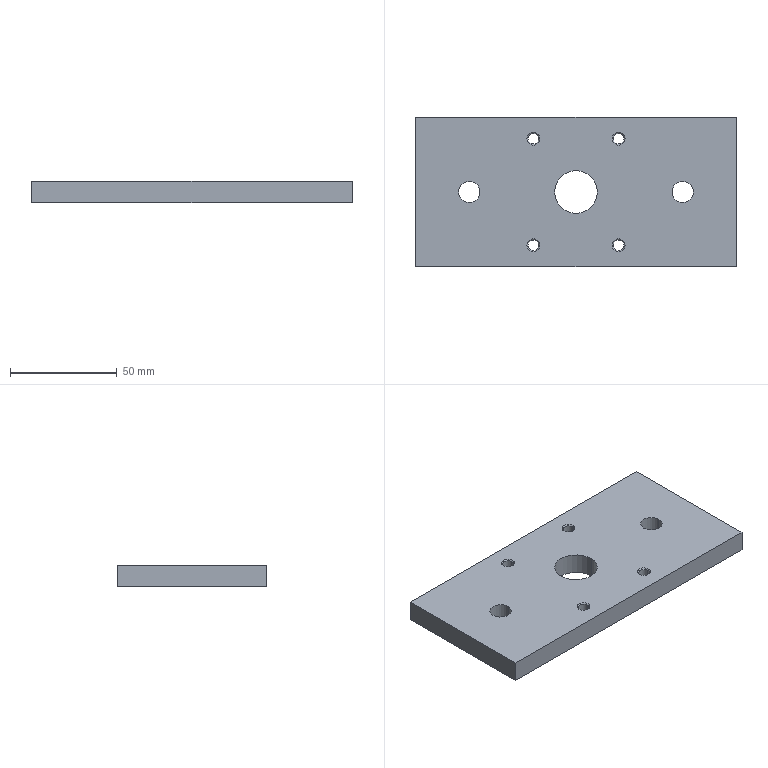Part | SolidWorks | features Cut 2, Extrusion 1, HoleWzd 1 | 1 solid | 28 faces | box 150 x 70 x 10 mm | volume 99493 mm3 | cylinder 14 | cone 8 | plane 6 | commonest cylinder face diameters 5 x8 10 x4 20 x2
STEP:
#1=CARTESIAN_POINT('',(17.5,25.,9.475));
#2=VERTEX_POINT('',#1);
#3=CARTESIAN_POINT('',(22.5,25.,9.475));
#4=VERTEX_POINT('',#3);
#5=CARTESIAN_POINT('',(20.,25.,9.475));
#6=DIRECTION('',(0.,0.,1.));
#7=DIRECTION('',(1.,0.,0.));
#8=AXIS2_PLACEMENT_3D('',#5,#6,#7);
#9=CIRCLE('',#8,2.5);
#10=EDGE_CURVE('',#2,#4,#9,.T.);
#11=ORIENTED_EDGE('',*,*,#10,.F.);
#12=CARTESIAN_POINT('',(16.975,25.,10.));
#13=VERTEX_POINT('',#12);
#14=CARTESIAN_POINT('',(16.975,25.,10.));
#15=DIRECTION('',(-0.7071,0.,0.7071));
#16=VECTOR('',#15,1000.);
#17=LINE('',#14,#16);
#18=EDGE_CURVE('',#2,#13,#17,.T.);
#19=ORIENTED_EDGE('',*,*,#18,.T.);
#20=CARTESIAN_POINT('',(23.025,25.,10.));
#21=VERTEX_POINT('',#20);
#22=CARTESIAN_POINT('',(20.,25.,10.));
#23=DIRECTION('',(0.,0.,1.));
#24=DIRECTION('',(1.,0.,0.));
#25=AXIS2_PLACEMENT_3D('',#22,#23,#24);
#26=CIRCLE('',#25,3.025);
#27=EDGE_CURVE('',#13,#21,#26,.T.);
#28=ORIENTED_EDGE('',*,*,#27,.T.);
#29=CARTESIAN_POINT('',(23.025,25.,10.));
#30=DIRECTION('',(0.7071,0.,0.7071));
#31=VECTOR('',#30,1000.);
#32=LINE('',#29,#31);
#33=EDGE_CURVE('',#4,#21,#32,.T.);
#34=ORIENTED_EDGE('',*,*,#33,.F.);
#35=EDGE_LOOP('',(#11,#19,#28,#34));
#36=FACE_OUTER_BOUND('',#35,.T.);
#37=CARTESIAN_POINT('',(20.,25.,10.));
#38=DIRECTION('',(0.,0.,1.));
#39=DIRECTION('',(1.,0.,0.));
#40=AXIS2_PLACEMENT_3D('',#37,#38,#39);
#41=CONICAL_SURFACE('',#40,3.025,0.7854);
#42=ADVANCED_FACE('',(#36),#41,.F.);
#43=CARTESIAN_POINT('',(17.5,25.,0.));
#44=VERTEX_POINT('',#43);
#45=CARTESIAN_POINT('',(22.5,25.,0.));
#46=VERTEX_POINT('',#45);
#47=CARTESIAN_POINT('',(20.,25.,0.));
#48=DIRECTION('',(0.,0.,1.));
#49=DIRECTION('',(1.,0.,0.));
#50=AXIS2_PLACEMENT_3D('',#47,#48,#49);
#51=CIRCLE('',#50,2.5);
#52=EDGE_CURVE('',#44,#46,#51,.T.);
#53=ORIENTED_EDGE('',*,*,#52,.F.);
#54=CARTESIAN_POINT('',(17.5,25.,10.));
#55=DIRECTION('',(0.,0.,1.));
#56=VECTOR('',#55,1000.);
#57=LINE('',#54,#56);
#58=EDGE_CURVE('',#44,#2,#57,.T.);
#59=ORIENTED_EDGE('',*,*,#58,.T.);
#60=ORIENTED_EDGE('',*,*,#10,.T.);
#61=CARTESIAN_POINT('',(22.5,25.,10.));
#62=DIRECTION('',(0.,0.,1.));
#63=VECTOR('',#62,1000.);
#64=LINE('',#61,#63);
#65=EDGE_CURVE('',#46,#4,#64,.T.);
#66=ORIENTED_EDGE('',*,*,#65,.F.);
#67=EDGE_LOOP('',(#53,#59,#60,#66));
#68=FACE_OUTER_BOUND('',#67,.T.);
#69=CARTESIAN_POINT('',(20.,25.,10.));
#70=DIRECTION('',(0.,0.,1.));
#71=DIRECTION('',(1.,0.,0.));
#72=AXIS2_PLACEMENT_3D('',#69,#70,#71);
#73=CYLINDRICAL_SURFACE('',#72,2.5);
#74=ADVANCED_FACE('',(#68),#73,.F.);
#75=CARTESIAN_POINT('',(-22.5,25.,9.475));
#76=VERTEX_POINT('',#75);
#77=CARTESIAN_POINT('',(-17.5,25.,9.475));
#78=VERTEX_POINT('',#77);
#79=CARTESIAN_POINT('',(-20.,25.,9.475));
#80=DIRECTION('',(0.,0.,1.));
#81=DIRECTION('',(1.,0.,0.));
#82=AXIS2_PLACEMENT_3D('',#79,#80,#81);
#83=CIRCLE('',#82,2.5);
#84=EDGE_CURVE('',#76,#78,#83,.T.);
#85=ORIENTED_EDGE('',*,*,#84,.F.);
#86=CARTESIAN_POINT('',(-23.025,25.,10.));
#87=VERTEX_POINT('',#86);
#88=CARTESIAN_POINT('',(-23.025,25.,10.));
#89=DIRECTION('',(-0.7071,0.,0.7071));
#90=VECTOR('',#89,1000.);
#91=LINE('',#88,#90);
#92=EDGE_CURVE('',#76,#87,#91,.T.);
#93=ORIENTED_EDGE('',*,*,#92,.T.);
#94=CARTESIAN_POINT('',(-16.975,25.,10.));
#95=VERTEX_POINT('',#94);
#96=CARTESIAN_POINT('',(-20.,25.,10.));
#97=DIRECTION('',(0.,0.,1.));
#98=DIRECTION('',(1.,0.,0.));
#99=AXIS2_PLACEMENT_3D('',#96,#97,#98);
#100=CIRCLE('',#99,3.025);
#101=EDGE_CURVE('',#87,#95,#100,.T.);
#102=ORIENTED_EDGE('',*,*,#101,.T.);
#103=CARTESIAN_POINT('',(-16.975,25.,10.));
#104=DIRECTION('',(0.7071,0.,0.7071));
#105=VECTOR('',#104,1000.);
#106=LINE('',#103,#105);
#107=EDGE_CURVE('',#78,#95,#106,.T.);
#108=ORIENTED_EDGE('',*,*,#107,.F.);
#109=EDGE_LOOP('',(#85,#93,#102,#108));
#110=FACE_OUTER_BOUND('',#109,.T.);
#111=CARTESIAN_POINT('',(-20.,25.,10.));
#112=DIRECTION('',(0.,0.,1.));
#113=DIRECTION('',(1.,0.,0.));
#114=AXIS2_PLACEMENT_3D('',#111,#112,#113);
#115=CONICAL_SURFACE('',#114,3.025,0.7854);
#116=ADVANCED_FACE('',(#110),#115,.F.);
#117=CARTESIAN_POINT('',(-22.5,25.,0.));
#118=VERTEX_POINT('',#117);
#119=CARTESIAN_POINT('',(-17.5,25.,0.));
#120=VERTEX_POINT('',#119);
#121=CARTESIAN_POINT('',(-20.,25.,0.));
#122=DIRECTION('',(0.,0.,1.));
#123=DIRECTION('',(1.,0.,0.));
#124=AXIS2_PLACEMENT_3D('',#121,#122,#123);
#125=CIRCLE('',#124,2.5);
#126=EDGE_CURVE('',#118,#120,#125,.T.);
#127=ORIENTED_EDGE('',*,*,#126,.F.);
#128=CARTESIAN_POINT('',(-22.5,25.,10.));
#129=DIRECTION('',(0.,0.,1.));
#130=VECTOR('',#129,1000.);
#131=LINE('',#128,#130);
#132=EDGE_CURVE('',#118,#76,#131,.T.);
#133=ORIENTED_EDGE('',*,*,#132,.T.);
#134=ORIENTED_EDGE('',*,*,#84,.T.);
#135=CARTESIAN_POINT('',(-17.5,25.,10.));
#136=DIRECTION('',(0.,0.,1.));
#137=VECTOR('',#136,1000.);
#138=LINE('',#135,#137);
#139=EDGE_CURVE('',#120,#78,#138,.T.);
#140=ORIENTED_EDGE('',*,*,#139,.F.);
#141=EDGE_LOOP('',(#127,#133,#134,#140));
#142=FACE_OUTER_BOUND('',#141,.T.);
#143=CARTESIAN_POINT('',(-20.,25.,10.));
#144=DIRECTION('',(0.,0.,1.));
#145=DIRECTION('',(1.,0.,0.));
#146=AXIS2_PLACEMENT_3D('',#143,#144,#145);
#147=CYLINDRICAL_SURFACE('',#146,2.5);
#148=ADVANCED_FACE('',(#142),#147,.F.);
#149=CARTESIAN_POINT('',(-22.5,-25.,9.475));
#150=VERTEX_POINT('',#149);
#151=CARTESIAN_POINT('',(-17.5,-25.,9.475));
#152=VERTEX_POINT('',#151);
#153=CARTESIAN_POINT('',(-20.,-25.,9.475));
#154=DIRECTION('',(0.,0.,1.));
#155=DIRECTION('',(1.,0.,0.));
#156=AXIS2_PLACEMENT_3D('',#153,#154,#155);
#157=CIRCLE('',#156,2.5);
#158=EDGE_CURVE('',#150,#152,#157,.T.);
#159=ORIENTED_EDGE('',*,*,#158,.F.);
#160=CARTESIAN_POINT('',(-23.025,-25.,10.));
#161=VERTEX_POINT('',#160);
#162=CARTESIAN_POINT('',(-23.025,-25.,10.));
#163=DIRECTION('',(-0.7071,0.,0.7071));
#164=VECTOR('',#163,1000.);
#165=LINE('',#162,#164);
#166=EDGE_CURVE('',#150,#161,#165,.T.);
#167=ORIENTED_EDGE('',*,*,#166,.T.);
#168=CARTESIAN_POINT('',(-16.975,-25.,10.));
#169=VERTEX_POINT('',#168);
#170=CARTESIAN_POINT('',(-20.,-25.,10.));
#171=DIRECTION('',(0.,0.,1.));
#172=DIRECTION('',(1.,0.,0.));
#173=AXIS2_PLACEMENT_3D('',#170,#171,#172);
#174=CIRCLE('',#173,3.025);
#175=EDGE_CURVE('',#161,#169,#174,.T.);
#176=ORIENTED_EDGE('',*,*,#175,.T.);
#177=CARTESIAN_POINT('',(-16.975,-25.,10.));
#178=DIRECTION('',(0.7071,0.,0.7071));
#179=VECTOR('',#178,1000.);
#180=LINE('',#177,#179);
#181=EDGE_CURVE('',#152,#169,#180,.T.);
#182=ORIENTED_EDGE('',*,*,#181,.F.);
#183=EDGE_LOOP('',(#159,#167,#176,#182));
#184=FACE_OUTER_BOUND('',#183,.T.);
#185=CARTESIAN_POINT('',(-20.,-25.,10.));
#186=DIRECTION('',(0.,0.,1.));
#187=DIRECTION('',(1.,0.,0.));
#188=AXIS2_PLACEMENT_3D('',#185,#186,#187);
#189=CONICAL_SURFACE('',#188,3.025,0.7854);
#190=ADVANCED_FACE('',(#184),#189,.F.);
#191=CARTESIAN_POINT('',(-22.5,-25.,0.));
#192=VERTEX_POINT('',#191);
#193=CARTESIAN_POINT('',(-17.5,-25.,0.));
#194=VERTEX_POINT('',#193);
#195=CARTESIAN_POINT('',(-20.,-25.,0.));
#196=DIRECTION('',(0.,0.,1.));
#197=DIRECTION('',(1.,0.,0.));
#198=AXIS2_PLACEMENT_3D('',#195,#196,#197);
#199=CIRCLE('',#198,2.5);
#200=EDGE_CURVE('',#192,#194,#199,.T.);
#201=ORIENTED_EDGE('',*,*,#200,.F.);
#202=CARTESIAN_POINT('',(-22.5,-25.,10.));
#203=DIRECTION('',(0.,0.,1.));
#204=VECTOR('',#203,1000.);
#205=LINE('',#202,#204);
#206=EDGE_CURVE('',#192,#150,#205,.T.);
#207=ORIENTED_EDGE('',*,*,#206,.T.);
#208=ORIENTED_EDGE('',*,*,#158,.T.);
#209=CARTESIAN_POINT('',(-17.5,-25.,10.));
#210=DIRECTION('',(0.,0.,1.));
#211=VECTOR('',#210,1000.);
#212=LINE('',#209,#211);
#213=EDGE_CURVE('',#194,#152,#212,.T.);
#214=ORIENTED_EDGE('',*,*,#213,.F.);
#215=EDGE_LOOP('',(#201,#207,#208,#214));
#216=FACE_OUTER_BOUND('',#215,.T.);
#217=CARTESIAN_POINT('',(-20.,-25.,10.));
#218=DIRECTION('',(0.,0.,1.));
#219=DIRECTION('',(1.,0.,0.));
#220=AXIS2_PLACEMENT_3D('',#217,#218,#219);
#221=CYLINDRICAL_SURFACE('',#220,2.5);
#222=ADVANCED_FACE('',(#216),#221,.F.);
#223=CARTESIAN_POINT('',(17.5,-25.,9.475));
#224=VERTEX_POINT('',#223);
#225=CARTESIAN_POINT('',(22.5,-25.,9.475));
#226=VERTEX_POINT('',#225);
#227=CARTESIAN_POINT('',(20.,-25.,9.475));
#228=DIRECTION('',(0.,0.,1.));
#229=DIRECTION('',(1.,0.,0.));
#230=AXIS2_PLACEMENT_3D('',#227,#228,#229);
#231=CIRCLE('',#230,2.5);
#232=EDGE_CURVE('',#224,#226,#231,.T.);
#233=ORIENTED_EDGE('',*,*,#232,.F.);
#234=CARTESIAN_POINT('',(16.975,-25.,10.));
#235=VERTEX_POINT('',#234);
#236=CARTESIAN_POINT('',(16.975,-25.,10.));
#237=DIRECTION('',(-0.7071,0.,0.7071));
#238=VECTOR('',#237,1000.);
#239=LINE('',#236,#238);
#240=EDGE_CURVE('',#224,#235,#239,.T.);
#241=ORIENTED_EDGE('',*,*,#240,.T.);
#242=CARTESIAN_POINT('',(23.025,-25.,10.));
#243=VERTEX_POINT('',#242);
#244=CARTESIAN_POINT('',(20.,-25.,10.));
#245=DIRECTION('',(0.,0.,1.));
#246=DIRECTION('',(1.,0.,0.));
#247=AXIS2_PLACEMENT_3D('',#244,#245,#246);
#248=CIRCLE('',#247,3.025);
#249=EDGE_CURVE('',#235,#243,#248,.T.);
#250=ORIENTED_EDGE('',*,*,#249,.T.);
#251=CARTESIAN_POINT('',(23.025,-25.,10.));
#252=DIRECTION('',(0.7071,0.,0.7071));
#253=VECTOR('',#252,1000.);
#254=LINE('',#251,#253);
#255=EDGE_CURVE('',#226,#243,#254,.T.);
#256=ORIENTED_EDGE('',*,*,#255,.F.);
#257=EDGE_LOOP('',(#233,#241,#250,#256));
#258=FACE_OUTER_BOUND('',#257,.T.);
#259=CARTESIAN_POINT('',(20.,-25.,10.));
#260=DIRECTION('',(0.,0.,1.));
#261=DIRECTION('',(1.,0.,0.));
#262=AXIS2_PLACEMENT_3D('',#259,#260,#261);
#263=CONICAL_SURFACE('',#262,3.025,0.7854);
#264=ADVANCED_FACE('',(#258),#263,.F.);
#265=CARTESIAN_POINT('',(17.5,-25.,0.));
#266=VERTEX_POINT('',#265);
#267=CARTESIAN_POINT('',(22.5,-25.,0.));
#268=VERTEX_POINT('',#267);
#269=CARTESIAN_POINT('',(20.,-25.,0.));
#270=DIRECTION('',(0.,0.,1.));
#271=DIRECTION('',(1.,0.,0.));
#272=AXIS2_PLACEMENT_3D('',#269,#270,#271);
#273=CIRCLE('',#272,2.5);
#274=EDGE_CURVE('',#266,#268,#273,.T.);
#275=ORIENTED_EDGE('',*,*,#274,.F.);
#276=CARTESIAN_POINT('',(17.5,-25.,10.));
#277=DIRECTION('',(0.,0.,1.));
#278=VECTOR('',#277,1000.);
#279=LINE('',#276,#278);
#280=EDGE_CURVE('',#266,#224,#279,.T.);
#281=ORIENTED_EDGE('',*,*,#280,.T.);
#282=ORIENTED_EDGE('',*,*,#232,.T.);
#283=CARTESIAN_POINT('',(22.5,-25.,10.));
#284=DIRECTION('',(0.,0.,1.));
#285=VECTOR('',#284,1000.);
#286=LINE('',#283,#285);
#287=EDGE_CURVE('',#268,#226,#286,.T.);
#288=ORIENTED_EDGE('',*,*,#287,.F.);
#289=EDGE_LOOP('',(#275,#281,#282,#288));
#290=FACE_OUTER_BOUND('',#289,.T.);
#291=CARTESIAN_POINT('',(20.,-25.,10.));
#292=DIRECTION('',(0.,0.,1.));
#293=DIRECTION('',(1.,0.,0.));
#294=AXIS2_PLACEMENT_3D('',#291,#292,#293);
#295=CYLINDRICAL_SURFACE('',#294,2.5);
#296=ADVANCED_FACE('',(#290),#295,.F.);
#297=CARTESIAN_POINT('',(-55.,0.,0.));
#298=VERTEX_POINT('',#297);
#299=CARTESIAN_POINT('',(-45.,0.,0.));
#300=VERTEX_POINT('',#299);
#301=CARTESIAN_POINT('',(-50.,0.,0.));
#302=DIRECTION('',(0.,0.,1.));
#303=DIRECTION('',(1.,0.,0.));
#304=AXIS2_PLACEMENT_3D('',#301,#302,#303);
#305=CIRCLE('',#304,5.);
#306=EDGE_CURVE('',#298,#300,#305,.T.);
#307=ORIENTED_EDGE('',*,*,#306,.F.);
#308=CARTESIAN_POINT('',(-55.,0.,10.));
#309=VERTEX_POINT('',#308);
#310=CARTESIAN_POINT('',(-55.,0.,-10.));
#311=DIRECTION('',(0.,0.,1.));
#312=VECTOR('',#311,1000.);
#313=LINE('',#310,#312);
#314=EDGE_CURVE('',#298,#309,#313,.T.);
#315=ORIENTED_EDGE('',*,*,#314,.T.);
#316=CARTESIAN_POINT('',(-45.,0.,10.));
#317=VERTEX_POINT('',#316);
#318=CARTESIAN_POINT('',(-50.,0.,10.));
#319=DIRECTION('',(0.,0.,1.));
#320=DIRECTION('',(1.,0.,0.));
#321=AXIS2_PLACEMENT_3D('',#318,#319,#320);
#322=CIRCLE('',#321,5.);
#323=EDGE_CURVE('',#309,#317,#322,.T.);
#324=ORIENTED_EDGE('',*,*,#323,.T.);
#325=CARTESIAN_POINT('',(-45.,0.,-10.));
#326=DIRECTION('',(0.,0.,1.));
#327=VECTOR('',#326,1000.);
#328=LINE('',#325,#327);
#329=EDGE_CURVE('',#300,#317,#328,.T.);
#330=ORIENTED_EDGE('',*,*,#329,.F.);
#331=EDGE_LOOP('',(#307,#315,#324,#330));
#332=FACE_OUTER_BOUND('',#331,.T.);
#333=CARTESIAN_POINT('',(-50.,0.,-10.));
#334=DIRECTION('',(0.,0.,1.));
#335=DIRECTION('',(1.,0.,0.));
#336=AXIS2_PLACEMENT_3D('',#333,#334,#335);
#337=CYLINDRICAL_SURFACE('',#336,5.);
#338=ADVANCED_FACE('',(#332),#337,.F.);
#339=CARTESIAN_POINT('',(45.,0.,0.));
#340=VERTEX_POINT('',#339);
#341=CARTESIAN_POINT('',(55.,0.,0.));
#342=VERTEX_POINT('',#341);
#343=CARTESIAN_POINT('',(50.,0.,0.));
#344=DIRECTION('',(0.,0.,1.));
#345=DIRECTION('',(1.,0.,0.));
#346=AXIS2_PLACEMENT_3D('',#343,#344,#345);
#347=CIRCLE('',#346,5.);
#348=EDGE_CURVE('',#340,#342,#347,.T.);
#349=ORIENTED_EDGE('',*,*,#348,.F.);
#350=CARTESIAN_POINT('',(45.,0.,10.));
#351=VERTEX_POINT('',#350);
#352=CARTESIAN_POINT('',(45.,0.,-10.));
#353=DIRECTION('',(0.,0.,1.));
#354=VECTOR('',#353,1000.);
#355=LINE('',#352,#354);
#356=EDGE_CURVE('',#340,#351,#355,.T.);
#357=ORIENTED_EDGE('',*,*,#356,.T.);
#358=CARTESIAN_POINT('',(55.,0.,10.));
#359=VERTEX_POINT('',#358);
#360=CARTESIAN_POINT('',(50.,0.,10.));
#361=DIRECTION('',(0.,0.,1.));
#362=DIRECTION('',(1.,0.,0.));
#363=AXIS2_PLACEMENT_3D('',#360,#361,#362);
#364=CIRCLE('',#363,5.);
#365=EDGE_CURVE('',#351,#359,#364,.T.);
#366=ORIENTED_EDGE('',*,*,#365,.T.);
#367=CARTESIAN_POINT('',(55.,0.,-10.));
#368=DIRECTION('',(0.,0.,1.));
#369=VECTOR('',#368,1000.);
#370=LINE('',#367,#369);
#371=EDGE_CURVE('',#342,#359,#370,.T.);
#372=ORIENTED_EDGE('',*,*,#371,.F.);
#373=EDGE_LOOP('',(#349,#357,#366,#372));
#374=FACE_OUTER_BOUND('',#373,.T.);
#375=CARTESIAN_POINT('',(50.,0.,-10.));
#376=DIRECTION('',(0.,0.,1.));
#377=DIRECTION('',(1.,0.,0.));
#378=AXIS2_PLACEMENT_3D('',#375,#376,#377);
#379=CYLINDRICAL_SURFACE('',#378,5.);
#380=ADVANCED_FACE('',(#374),#379,.F.);
#381=CARTESIAN_POINT('',(-10.,0.,0.));
#382=VERTEX_POINT('',#381);
#383=CARTESIAN_POINT('',(10.,0.,0.));
#384=VERTEX_POINT('',#383);
#385=CARTESIAN_POINT('',(0.,0.,0.));
#386=DIRECTION('',(0.,0.,1.));
#387=DIRECTION('',(1.,0.,0.));
#388=AXIS2_PLACEMENT_3D('',#385,#386,#387);
#389=CIRCLE('',#388,10.);
#390=EDGE_CURVE('',#382,#384,#389,.T.);
#391=ORIENTED_EDGE('',*,*,#390,.F.);
#392=CARTESIAN_POINT('',(-10.,0.,10.));
#393=VERTEX_POINT('',#392);
#394=CARTESIAN_POINT('',(-10.,0.,-45.));
#395=DIRECTION('',(0.,0.,1.));
#396=VECTOR('',#395,1000.);
#397=LINE('',#394,#396);
#398=EDGE_CURVE('',#382,#393,#397,.T.);
#399=ORIENTED_EDGE('',*,*,#398,.T.);
#400=CARTESIAN_POINT('',(10.,0.,10.));
#401=VERTEX_POINT('',#400);
#402=CARTESIAN_POINT('',(0.,0.,10.));
#403=DIRECTION('',(0.,0.,1.));
#404=DIRECTION('',(1.,0.,0.));
#405=AXIS2_PLACEMENT_3D('',#402,#403,#404);
#406=CIRCLE('',#405,10.);
#407=EDGE_CURVE('',#393,#401,#406,.T.);
#408=ORIENTED_EDGE('',*,*,#407,.T.);
#409=CARTESIAN_POINT('',(10.,0.,-45.));
#410=DIRECTION('',(0.,0.,1.));
#411=VECTOR('',#410,1000.);
#412=LINE('',#409,#411);
#413=EDGE_CURVE('',#384,#401,#412,.T.);
#414=ORIENTED_EDGE('',*,*,#413,.F.);
#415=EDGE_LOOP('',(#391,#399,#408,#414));
#416=FACE_OUTER_BOUND('',#415,.T.);
#417=CARTESIAN_POINT('',(0.,0.,-45.));
#418=DIRECTION('',(0.,0.,1.));
#419=DIRECTION('',(1.,0.,0.));
#420=AXIS2_PLACEMENT_3D('',#417,#418,#419);
#421=CYLINDRICAL_SURFACE('',#420,10.);
#422=ADVANCED_FACE('',(#416),#421,.F.);
#423=CARTESIAN_POINT('',(75.,-35.,0.));
#424=VERTEX_POINT('',#423);
#425=CARTESIAN_POINT('',(75.,35.,0.));
#426=VERTEX_POINT('',#425);
#427=CARTESIAN_POINT('',(75.,35.,0.));
#428=DIRECTION('',(0.,1.,0.));
#429=VECTOR('',#428,1000.);
#430=LINE('',#427,#429);
#431=EDGE_CURVE('',#424,#426,#430,.T.);
#432=ORIENTED_EDGE('',*,*,#431,.T.);
#433=CARTESIAN_POINT('',(75.,35.,10.));
#434=VERTEX_POINT('',#433);
#435=CARTESIAN_POINT('',(75.,35.,10.));
#436=DIRECTION('',(0.,0.,-1.));
#437=VECTOR('',#436,1000.);
#438=LINE('',#435,#437);
#439=EDGE_CURVE('',#434,#426,#438,.T.);
#440=ORIENTED_EDGE('',*,*,#439,.F.);
#441=CARTESIAN_POINT('',(75.,-35.,10.));
#442=VERTEX_POINT('',#441);
#443=CARTESIAN_POINT('',(75.,35.,10.));
#444=DIRECTION('',(0.,1.,0.));
#445=VECTOR('',#444,1000.);
#446=LINE('',#443,#445);
#447=EDGE_CURVE('',#442,#434,#446,.T.);
#448=ORIENTED_EDGE('',*,*,#447,.F.);
#449=CARTESIAN_POINT('',(75.,-35.,10.));
#450=DIRECTION('',(0.,0.,-1.));
#451=VECTOR('',#450,1000.);
#452=LINE('',#449,#451);
#453=EDGE_CURVE('',#442,#424,#452,.T.);
#454=ORIENTED_EDGE('',*,*,#453,.T.);
#455=EDGE_LOOP('',(#432,#440,#448,#454));
#456=FACE_OUTER_BOUND('',#455,.T.);
#457=CARTESIAN_POINT('',(75.,35.,10.));
#458=DIRECTION('',(-1.,0.,0.));
#459=DIRECTION('',(0.,0.,1.));
#460=AXIS2_PLACEMENT_3D('',#457,#458,#459);
#461=PLANE('',#460);
#462=ADVANCED_FACE('',(#456),#461,.F.);
#463=CARTESIAN_POINT('',(-75.,35.,0.));
#464=VERTEX_POINT('',#463);
#465=CARTESIAN_POINT('',(-75.,35.,0.));
#466=DIRECTION('',(-1.,0.,0.));
#467=VECTOR('',#466,1000.);
#468=LINE('',#465,#467);
#469=EDGE_CURVE('',#426,#464,#468,.T.);
#470=ORIENTED_EDGE('',*,*,#469,.T.);
#471=CARTESIAN_POINT('',(-75.,35.,10.));
#472=VERTEX_POINT('',#471);
#473=CARTESIAN_POINT('',(-75.,35.,10.));
#474=DIRECTION('',(0.,0.,-1.));
#475=VECTOR('',#474,1000.);
#476=LINE('',#473,#475);
#477=EDGE_CURVE('',#472,#464,#476,.T.);
#478=ORIENTED_EDGE('',*,*,#477,.F.);
#479=CARTESIAN_POINT('',(-75.,35.,10.));
#480=DIRECTION('',(-1.,0.,0.));
#481=VECTOR('',#480,1000.);
#482=LINE('',#479,#481);
#483=EDGE_CURVE('',#434,#472,#482,.T.);
#484=ORIENTED_EDGE('',*,*,#483,.F.);
#485=ORIENTED_EDGE('',*,*,#439,.T.);
#486=EDGE_LOOP('',(#470,#478,#484,#485));
#487=FACE_OUTER_BOUND('',#486,.T.);
#488=CARTESIAN_POINT('',(-75.,35.,10.));
#489=DIRECTION('',(0.,-1.,0.));
#490=DIRECTION('',(0.,0.,-1.));
#491=AXIS2_PLACEMENT_3D('',#488,#489,#490);
#492=PLANE('',#491);
#493=ADVANCED_FACE('',(#487),#492,.F.);
#494=CARTESIAN_POINT('',(-75.,-35.,0.));
#495=VERTEX_POINT('',#494);
#496=CARTESIAN_POINT('',(-75.,35.,0.));
#497=DIRECTION('',(0.,-1.,0.));
#498=VECTOR('',#497,1000.);
#499=LINE('',#496,#498);
#500=EDGE_CURVE('',#464,#495,#499,.T.);
#501=ORIENTED_EDGE('',*,*,#500,.T.);
#502=CARTESIAN_POINT('',(-75.,-35.,10.));
#503=VERTEX_POINT('',#502);
#504=CARTESIAN_POINT('',(-75.,-35.,10.));
#505=DIRECTION('',(0.,0.,-1.));
#506=VECTOR('',#505,1000.);
#507=LINE('',#504,#506);
#508=EDGE_CURVE('',#503,#495,#507,.T.);
#509=ORIENTED_EDGE('',*,*,#508,.F.);
#510=CARTESIAN_POINT('',(-75.,35.,10.));
#511=DIRECTION('',(0.,-1.,0.));
#512=VECTOR('',#511,1000.);
#513=LINE('',#510,#512);
#514=EDGE_CURVE('',#472,#503,#513,.T.);
#515=ORIENTED_EDGE('',*,*,#514,.F.);
#516=ORIENTED_EDGE('',*,*,#477,.T.);
#517=EDGE_LOOP('',(#501,#509,#515,#516));
#518=FACE_OUTER_BOUND('',#517,.T.);
#519=CARTESIAN_POINT('',(-75.,35.,10.));
#520=DIRECTION('',(1.,0.,0.));
#521=DIRECTION('',(0.,1.,0.));
#522=AXIS2_PLACEMENT_3D('',#519,#520,#521);
#523=PLANE('',#522);
#524=ADVANCED_FACE('',(#518),#523,.F.);
#525=CARTESIAN_POINT('',(-75.,-35.,0.));
#526=DIRECTION('',(1.,0.,0.));
#527=VECTOR('',#526,1000.);
#528=LINE('',#525,#527);
#529=EDGE_CURVE('',#495,#424,#528,.T.);
#530=ORIENTED_EDGE('',*,*,#529,.T.);
#531=ORIENTED_EDGE('',*,*,#453,.F.);
#532=CARTESIAN_POINT('',(-75.,-35.,10.));
#533=DIRECTION('',(1.,0.,0.));
#534=VECTOR('',#533,1000.);
#535=LINE('',#532,#534);
#536=EDGE_CURVE('',#503,#442,#535,.T.);
#537=ORIENTED_EDGE('',*,*,#536,.F.);
#538=ORIENTED_EDGE('',*,*,#508,.T.);
#539=EDGE_LOOP('',(#530,#531,#537,#538));
#540=FACE_OUTER_BOUND('',#539,.T.);
#541=CARTESIAN_POINT('',(-75.,-35.,10.));
#542=DIRECTION('',(0.,1.,0.));
#543=DIRECTION('',(0.,0.,1.));
#544=AXIS2_PLACEMENT_3D('',#541,#542,#543);
#545=PLANE('',#544);
#546=ADVANCED_FACE('',(#540),#545,.F.);
#547=CARTESIAN_POINT('',(20.,25.,10.));
#548=DIRECTION('',(0.,0.,1.));
#549=DIRECTION('',(1.,0.,0.));
#550=AXIS2_PLACEMENT_3D('',#547,#548,#549);
#551=CIRCLE('',#550,3.025);
#552=EDGE_CURVE('',#21,#13,#551,.T.);
#553=ORIENTED_EDGE('',*,*,#552,.F.);
#554=ORIENTED_EDGE('',*,*,#27,.F.);
#555=EDGE_LOOP('',(#553,#554));
#556=FACE_BOUND('',#555,.T.);
#557=CARTESIAN_POINT('',(-20.,25.,10.));
#558=DIRECTION('',(0.,0.,1.));
#559=DIRECTION('',(1.,0.,0.));
#560=AXIS2_PLACEMENT_3D('',#557,#558,#559);
#561=CIRCLE('',#560,3.025);
#562=EDGE_CURVE('',#95,#87,#561,.T.);
#563=ORIENTED_EDGE('',*,*,#562,.F.);
#564=ORIENTED_EDGE('',*,*,#101,.F.);
#565=EDGE_LOOP('',(#563,#564));
#566=FACE_BOUND('',#565,.T.);
#567=CARTESIAN_POINT('',(-20.,-25.,10.));
#568=DIRECTION('',(0.,0.,1.));
#569=DIRECTION('',(1.,0.,0.));
#570=AXIS2_PLACEMENT_3D('',#567,#568,#569);
#571=CIRCLE('',#570,3.025);
#572=EDGE_CURVE('',#169,#161,#571,.T.);
#573=ORIENTED_EDGE('',*,*,#572,.F.);
#574=ORIENTED_EDGE('',*,*,#175,.F.);
#575=EDGE_LOOP('',(#573,#574));
#576=FACE_BOUND('',#575,.T.);
#577=CARTESIAN_POINT('',(20.,-25.,10.));
#578=DIRECTION('',(0.,0.,1.));
#579=DIRECTION('',(1.,0.,0.));
#580=AXIS2_PLACEMENT_3D('',#577,#578,#579);
#581=CIRCLE('',#580,3.025);
#582=EDGE_CURVE('',#243,#235,#581,.T.);
#583=ORIENTED_EDGE('',*,*,#582,.F.);
#584=ORIENTED_EDGE('',*,*,#249,.F.);
#585=EDGE_LOOP('',(#583,#584));
#586=FACE_BOUND('',#585,.T.);
#587=CARTESIAN_POINT('',(-50.,0.,10.));
#588=DIRECTION('',(0.,0.,1.));
#589=DIRECTION('',(1.,0.,0.));
#590=AXIS2_PLACEMENT_3D('',#587,#588,#589);
#591=CIRCLE('',#590,5.);
#592=EDGE_CURVE('',#317,#309,#591,.T.);
#593=ORIENTED_EDGE('',*,*,#592,.F.);
#594=ORIENTED_EDGE('',*,*,#323,.F.);
#595=EDGE_LOOP('',(#593,#594));
#596=FACE_BOUND('',#595,.T.);
#597=CARTESIAN_POINT('',(50.,0.,10.));
#598=DIRECTION('',(0.,0.,1.));
#599=DIRECTION('',(1.,0.,0.));
#600=AXIS2_PLACEMENT_3D('',#597,#598,#599);
#601=CIRCLE('',#600,5.);
#602=EDGE_CURVE('',#359,#351,#601,.T.);
#603=ORIENTED_EDGE('',*,*,#602,.F.);
#604=ORIENTED_EDGE('',*,*,#365,.F.);
#605=EDGE_LOOP('',(#603,#604));
#606=FACE_BOUND('',#605,.T.);
#607=CARTESIAN_POINT('',(0.,0.,10.));
#608=DIRECTION('',(0.,0.,1.));
#609=DIRECTION('',(1.,0.,0.));
#610=AXIS2_PLACEMENT_3D('',#607,#608,#609);
#611=CIRCLE('',#610,10.);
#612=EDGE_CURVE('',#401,#393,#611,.T.);
#613=ORIENTED_EDGE('',*,*,#612,.F.);
#614=ORIENTED_EDGE('',*,*,#407,.F.);
#615=EDGE_LOOP('',(#613,#614));
#616=FACE_BOUND('',#615,.T.);
#617=ORIENTED_EDGE('',*,*,#447,.T.);
#618=ORIENTED_EDGE('',*,*,#483,.T.);
#619=ORIENTED_EDGE('',*,*,#514,.T.);
#620=ORIENTED_EDGE('',*,*,#536,.T.);
#621=EDGE_LOOP('',(#617,#618,#619,#620));
#622=FACE_OUTER_BOUND('',#621,.T.);
#623=CARTESIAN_POINT('',(0.,0.,10.));
#624=DIRECTION('',(0.,0.,1.));
#625=DIRECTION('',(1.,0.,0.));
#626=AXIS2_PLACEMENT_3D('',#623,#624,#625);
#627=PLANE('',#626);
#628=ADVANCED_FACE('',(#556,#566,#576,#586,#596,#606,#616,#622),#627,.T.);
#629=CARTESIAN_POINT('',(20.,25.,0.));
#630=DIRECTION('',(0.,0.,1.));
#631=DIRECTION('',(1.,0.,0.));
#632=AXIS2_PLACEMENT_3D('',#629,#630,#631);
#633=CIRCLE('',#632,2.5);
#634=EDGE_CURVE('',#46,#44,#633,.T.);
#635=ORIENTED_EDGE('',*,*,#634,.T.);
#636=ORIENTED_EDGE('',*,*,#52,.T.);
#637=EDGE_LOOP('',(#635,#636));
#638=FACE_BOUND('',#637,.T.);
#639=CARTESIAN_POINT('',(-20.,25.,0.));
#640=DIRECTION('',(0.,0.,1.));
#641=DIRECTION('',(1.,0.,0.));
#642=AXIS2_PLACEMENT_3D('',#639,#640,#641);
#643=CIRCLE('',#642,2.5);
#644=EDGE_CURVE('',#120,#118,#643,.T.);
#645=ORIENTED_EDGE('',*,*,#644,.T.);
#646=ORIENTED_EDGE('',*,*,#126,.T.);
#647=EDGE_LOOP('',(#645,#646));
#648=FACE_BOUND('',#647,.T.);
#649=CARTESIAN_POINT('',(-20.,-25.,0.));
#650=DIRECTION('',(0.,0.,1.));
#651=DIRECTION('',(1.,0.,0.));
#652=AXIS2_PLACEMENT_3D('',#649,#650,#651);
#653=CIRCLE('',#652,2.5);
#654=EDGE_CURVE('',#194,#192,#653,.T.);
#655=ORIENTED_EDGE('',*,*,#654,.T.);
#656=ORIENTED_EDGE('',*,*,#200,.T.);
#657=EDGE_LOOP('',(#655,#656));
#658=FACE_BOUND('',#657,.T.);
#659=CARTESIAN_POINT('',(20.,-25.,0.));
#660=DIRECTION('',(0.,0.,1.));
#661=DIRECTION('',(1.,0.,0.));
#662=AXIS2_PLACEMENT_3D('',#659,#660,#661);
#663=CIRCLE('',#662,2.5);
#664=EDGE_CURVE('',#268,#266,#663,.T.);
#665=ORIENTED_EDGE('',*,*,#664,.T.);
#666=ORIENTED_EDGE('',*,*,#274,.T.);
#667=EDGE_LOOP('',(#665,#666));
#668=FACE_BOUND('',#667,.T.);
#669=CARTESIAN_POINT('',(-50.,0.,0.));
#670=DIRECTION('',(0.,0.,1.));
#671=DIRECTION('',(1.,0.,0.));
#672=AXIS2_PLACEMENT_3D('',#669,#670,#671);
#673=CIRCLE('',#672,5.);
#674=EDGE_CURVE('',#300,#298,#673,.T.);
#675=ORIENTED_EDGE('',*,*,#674,.T.);
#676=ORIENTED_EDGE('',*,*,#306,.T.);
#677=EDGE_LOOP('',(#675,#676));
#678=FACE_BOUND('',#677,.T.);
#679=CARTESIAN_POINT('',(50.,0.,0.));
#680=DIRECTION('',(0.,0.,1.));
#681=DIRECTION('',(1.,0.,0.));
#682=AXIS2_PLACEMENT_3D('',#679,#680,#681);
#683=CIRCLE('',#682,5.);
#684=EDGE_CURVE('',#342,#340,#683,.T.);
#685=ORIENTED_EDGE('',*,*,#684,.T.);
#686=ORIENTED_EDGE('',*,*,#348,.T.);
#687=EDGE_LOOP('',(#685,#686));
#688=FACE_BOUND('',#687,.T.);
#689=CARTESIAN_POINT('',(0.,0.,0.));
#690=DIRECTION('',(0.,0.,1.));
#691=DIRECTION('',(1.,0.,0.));
#692=AXIS2_PLACEMENT_3D('',#689,#690,#691);
#693=CIRCLE('',#692,10.);
#694=EDGE_CURVE('',#384,#382,#693,.T.);
#695=ORIENTED_EDGE('',*,*,#694,.T.);
#696=ORIENTED_EDGE('',*,*,#390,.T.);
#697=EDGE_LOOP('',(#695,#696));
#698=FACE_BOUND('',#697,.T.);
#699=ORIENTED_EDGE('',*,*,#431,.F.);
#700=ORIENTED_EDGE('',*,*,#529,.F.);
#701=ORIENTED_EDGE('',*,*,#500,.F.);
#702=ORIENTED_EDGE('',*,*,#469,.F.);
#703=EDGE_LOOP('',(#699,#700,#701,#702));
#704=FACE_OUTER_BOUND('',#703,.T.);
#705=CARTESIAN_POINT('',(0.,0.,0.));
#706=DIRECTION('',(0.,0.,1.));
#707=DIRECTION('',(1.,0.,0.));
#708=AXIS2_PLACEMENT_3D('',#705,#706,#707);
#709=PLANE('',#708);
#710=ADVANCED_FACE('',(#638,#648,#658,#668,#678,#688,#698,#704),#709,.F.);
#711=ORIENTED_EDGE('',*,*,#398,.F.);
#712=ORIENTED_EDGE('',*,*,#694,.F.);
#713=ORIENTED_EDGE('',*,*,#413,.T.);
#714=ORIENTED_EDGE('',*,*,#612,.T.);
#715=EDGE_LOOP('',(#711,#712,#713,#714));
#716=FACE_OUTER_BOUND('',#715,.T.);
#717=CARTESIAN_POINT('',(0.,0.,-45.));
#718=DIRECTION('',(0.,0.,1.));
#719=DIRECTION('',(1.,0.,0.));
#720=AXIS2_PLACEMENT_3D('',#717,#718,#719);
#721=CYLINDRICAL_SURFACE('',#720,10.);
#722=ADVANCED_FACE('',(#716),#721,.F.);
#723=ORIENTED_EDGE('',*,*,#356,.F.);
#724=ORIENTED_EDGE('',*,*,#684,.F.);
#725=ORIENTED_EDGE('',*,*,#371,.T.);
#726=ORIENTED_EDGE('',*,*,#602,.T.);
#727=EDGE_LOOP('',(#723,#724,#725,#726));
#728=FACE_OUTER_BOUND('',#727,.T.);
#729=CARTESIAN_POINT('',(50.,0.,-10.));
#730=DIRECTION('',(0.,0.,1.));
#731=DIRECTION('',(1.,0.,0.));
#732=AXIS2_PLACEMENT_3D('',#729,#730,#731);
#733=CYLINDRICAL_SURFACE('',#732,5.);
#734=ADVANCED_FACE('',(#728),#733,.F.);
#735=ORIENTED_EDGE('',*,*,#314,.F.);
#736=ORIENTED_EDGE('',*,*,#674,.F.);
#737=ORIENTED_EDGE('',*,*,#329,.T.);
#738=ORIENTED_EDGE('',*,*,#592,.T.);
#739=EDGE_LOOP('',(#735,#736,#737,#738));
#740=FACE_OUTER_BOUND('',#739,.T.);
#741=CARTESIAN_POINT('',(-50.,0.,-10.));
#742=DIRECTION('',(0.,0.,1.));
#743=DIRECTION('',(1.,0.,0.));
#744=AXIS2_PLACEMENT_3D('',#741,#742,#743);
#745=CYLINDRICAL_SURFACE('',#744,5.);
#746=ADVANCED_FACE('',(#740),#745,.F.);
#747=ORIENTED_EDGE('',*,*,#280,.F.);
#748=ORIENTED_EDGE('',*,*,#664,.F.);
#749=ORIENTED_EDGE('',*,*,#287,.T.);
#750=CARTESIAN_POINT('',(20.,-25.,9.475));
#751=DIRECTION('',(0.,0.,1.));
#752=DIRECTION('',(1.,0.,0.));
#753=AXIS2_PLACEMENT_3D('',#750,#751,#752);
#754=CIRCLE('',#753,2.5);
#755=EDGE_CURVE('',#226,#224,#754,.T.);
#756=ORIENTED_EDGE('',*,*,#755,.T.);
#757=EDGE_LOOP('',(#747,#748,#749,#756));
#758=FACE_OUTER_BOUND('',#757,.T.);
#759=CARTESIAN_POINT('',(20.,-25.,10.));
#760=DIRECTION('',(0.,0.,1.));
#761=DIRECTION('',(1.,0.,0.));
#762=AXIS2_PLACEMENT_3D('',#759,#760,#761);
#763=CYLINDRICAL_SURFACE('',#762,2.5);
#764=ADVANCED_FACE('',(#758),#763,.F.);
#765=ORIENTED_EDGE('',*,*,#240,.F.);
#766=ORIENTED_EDGE('',*,*,#755,.F.);
#767=ORIENTED_EDGE('',*,*,#255,.T.);
#768=ORIENTED_EDGE('',*,*,#582,.T.);
#769=EDGE_LOOP('',(#765,#766,#767,#768));
#770=FACE_OUTER_BOUND('',#769,.T.);
#771=CARTESIAN_POINT('',(20.,-25.,10.));
#772=DIRECTION('',(0.,0.,1.));
#773=DIRECTION('',(1.,0.,0.));
#774=AXIS2_PLACEMENT_3D('',#771,#772,#773);
#775=CONICAL_SURFACE('',#774,3.025,0.7854);
#776=ADVANCED_FACE('',(#770),#775,.F.);
#777=ORIENTED_EDGE('',*,*,#206,.F.);
#778=ORIENTED_EDGE('',*,*,#654,.F.);
#779=ORIENTED_EDGE('',*,*,#213,.T.);
#780=CARTESIAN_POINT('',(-20.,-25.,9.475));
#781=DIRECTION('',(0.,0.,1.));
#782=DIRECTION('',(1.,0.,0.));
#783=AXIS2_PLACEMENT_3D('',#780,#781,#782);
#784=CIRCLE('',#783,2.5);
#785=EDGE_CURVE('',#152,#150,#784,.T.);
#786=ORIENTED_EDGE('',*,*,#785,.T.);
#787=EDGE_LOOP('',(#777,#778,#779,#786));
#788=FACE_OUTER_BOUND('',#787,.T.);
#789=CARTESIAN_POINT('',(-20.,-25.,10.));
#790=DIRECTION('',(0.,0.,1.));
#791=DIRECTION('',(1.,0.,0.));
#792=AXIS2_PLACEMENT_3D('',#789,#790,#791);
#793=CYLINDRICAL_SURFACE('',#792,2.5);
#794=ADVANCED_FACE('',(#788),#793,.F.);
#795=ORIENTED_EDGE('',*,*,#166,.F.);
#796=ORIENTED_EDGE('',*,*,#785,.F.);
#797=ORIENTED_EDGE('',*,*,#181,.T.);
#798=ORIENTED_EDGE('',*,*,#572,.T.);
#799=EDGE_LOOP('',(#795,#796,#797,#798));
#800=FACE_OUTER_BOUND('',#799,.T.);
#801=CARTESIAN_POINT('',(-20.,-25.,10.));
#802=DIRECTION('',(0.,0.,1.));
#803=DIRECTION('',(1.,0.,0.));
#804=AXIS2_PLACEMENT_3D('',#801,#802,#803);
#805=CONICAL_SURFACE('',#804,3.025,0.7854);
#806=ADVANCED_FACE('',(#800),#805,.F.);
#807=ORIENTED_EDGE('',*,*,#132,.F.);
#808=ORIENTED_EDGE('',*,*,#644,.F.);
#809=ORIENTED_EDGE('',*,*,#139,.T.);
#810=CARTESIAN_POINT('',(-20.,25.,9.475));
#811=DIRECTION('',(0.,0.,1.));
#812=DIRECTION('',(1.,0.,0.));
#813=AXIS2_PLACEMENT_3D('',#810,#811,#812);
#814=CIRCLE('',#813,2.5);
#815=EDGE_CURVE('',#78,#76,#814,.T.);
#816=ORIENTED_EDGE('',*,*,#815,.T.);
#817=EDGE_LOOP('',(#807,#808,#809,#816));
#818=FACE_OUTER_BOUND('',#817,.T.);
#819=CARTESIAN_POINT('',(-20.,25.,10.));
#820=DIRECTION('',(0.,0.,1.));
#821=DIRECTION('',(1.,0.,0.));
#822=AXIS2_PLACEMENT_3D('',#819,#820,#821);
#823=CYLINDRICAL_SURFACE('',#822,2.5);
#824=ADVANCED_FACE('',(#818),#823,.F.);
#825=ORIENTED_EDGE('',*,*,#92,.F.);
#826=ORIENTED_EDGE('',*,*,#815,.F.);
#827=ORIENTED_EDGE('',*,*,#107,.T.);
#828=ORIENTED_EDGE('',*,*,#562,.T.);
#829=EDGE_LOOP('',(#825,#826,#827,#828));
#830=FACE_OUTER_BOUND('',#829,.T.);
#831=CARTESIAN_POINT('',(-20.,25.,10.));
#832=DIRECTION('',(0.,0.,1.));
#833=DIRECTION('',(1.,0.,0.));
#834=AXIS2_PLACEMENT_3D('',#831,#832,#833);
#835=CONICAL_SURFACE('',#834,3.025,0.7854);
#836=ADVANCED_FACE('',(#830),#835,.F.);
#837=ORIENTED_EDGE('',*,*,#58,.F.);
#838=ORIENTED_EDGE('',*,*,#634,.F.);
#839=ORIENTED_EDGE('',*,*,#65,.T.);
#840=CARTESIAN_POINT('',(20.,25.,9.475));
#841=DIRECTION('',(0.,0.,1.));
#842=DIRECTION('',(1.,0.,0.));
#843=AXIS2_PLACEMENT_3D('',#840,#841,#842);
#844=CIRCLE('',#843,2.5);
#845=EDGE_CURVE('',#4,#2,#844,.T.);
#846=ORIENTED_EDGE('',*,*,#845,.T.);
#847=EDGE_LOOP('',(#837,#838,#839,#846));
#848=FACE_OUTER_BOUND('',#847,.T.);
#849=CARTESIAN_POINT('',(20.,25.,10.));
#850=DIRECTION('',(0.,0.,1.));
#851=DIRECTION('',(1.,0.,0.));
#852=AXIS2_PLACEMENT_3D('',#849,#850,#851);
#853=CYLINDRICAL_SURFACE('',#852,2.5);
#854=ADVANCED_FACE('',(#848),#853,.F.);
#855=ORIENTED_EDGE('',*,*,#18,.F.);
#856=ORIENTED_EDGE('',*,*,#845,.F.);
#857=ORIENTED_EDGE('',*,*,#33,.T.);
#858=ORIENTED_EDGE('',*,*,#552,.T.);
#859=EDGE_LOOP('',(#855,#856,#857,#858));
#860=FACE_OUTER_BOUND('',#859,.T.);
#861=CARTESIAN_POINT('',(20.,25.,10.));
#862=DIRECTION('',(0.,0.,1.));
#863=DIRECTION('',(1.,0.,0.));
#864=AXIS2_PLACEMENT_3D('',#861,#862,#863);
#865=CONICAL_SURFACE('',#864,3.025,0.7854);
#866=ADVANCED_FACE('',(#860),#865,.F.);
#867=CLOSED_SHELL('',(#42,#74,#116,#148,#190,#222,#264,#296,#338,#380,#422,#462,#493,#524,#546,#628,#710,#722,#734,#746,#764,#776,#794,#806,#824,#836,#854,#866));
#868=MANIFOLD_SOLID_BREP('',#867);
#869=CARTESIAN_POINT('',(0.,0.,0.));
#870=DIRECTION('',(0.,0.,1.));
#871=DIRECTION('',(1.,0.,0.));
#872=AXIS2_PLACEMENT_3D('',#869,#870,#871);
#873=(LENGTH_UNIT()NAMED_UNIT(*)SI_UNIT(.MILLI.,.METRE.));
#874=UNCERTAINTY_MEASURE_WITH_UNIT(LENGTH_MEASURE(0.00001),#873,'','');
#875=(NAMED_UNIT(*)PLANE_ANGLE_UNIT()SI_UNIT($,.RADIAN.));
#876=(NAMED_UNIT(*)SI_UNIT($,.STERADIAN.)SOLID_ANGLE_UNIT());
#877=(GEOMETRIC_REPRESENTATION_CONTEXT(3)GLOBAL_UNCERTAINTY_ASSIGNED_CONTEXT((#874))GLOBAL_UNIT_ASSIGNED_CONTEXT((#873,#875,#876))REPRESENTATION_CONTEXT('',''));
#878=ADVANCED_BREP_SHAPE_REPRESENTATION('',(#868,#872),#877);